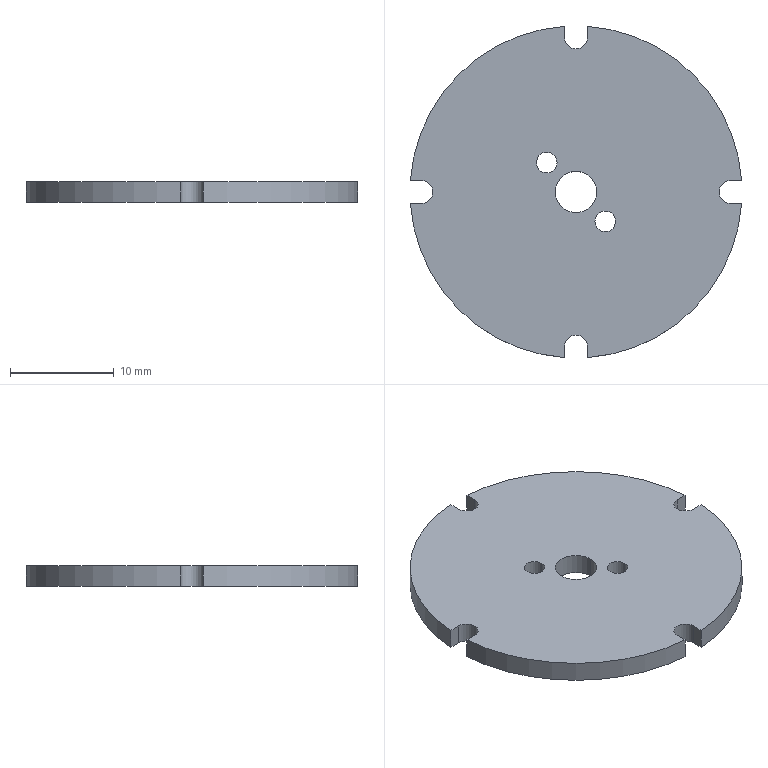Part | STEP file | ASND-0110-SDS_6 | 1 solid | 24 faces | box 31.924 x 31.924 x 2 mm | volume 1536 mm3 | cylinder 14 | plane 10 | commonest cylinder face diameters 2 x4 2.2 x4 32 x4 4 x2